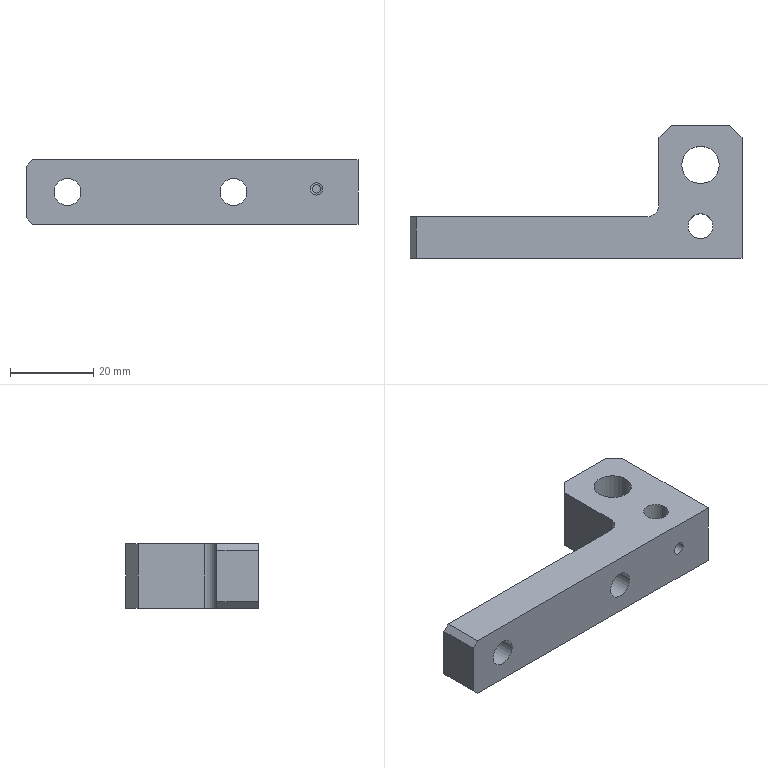NC program | NX | posted with a generic post | part box 80 x 32 x 15.5 mm
Lines 1 to 1192 of 7013:
N10 G17 G21 G94 G90
(低壁铣光面 , TOOL : D63面刀)
N12 T10 M6
N14 G53
N16 G17 G0 G90 X74.5 Y-0.25 B0. C0. S1600 M3
N18 G43 Z20. H10
N20 Z3.
N22 G94 G1 Z0. F500.
N24 X71.5
N26 X-70.
N28 X-73.
N30 Z3.
N32 G0 Z20.
N34 M5
(动态粗 , TOOL : D10-30-D10-75-3T-ROUGH)
N36 T01 M6
N38 G53
N40 G17 G0 G90 X49.529 Y17.135 B0. C0. S3500 M3
N42 G43 Z20. H1
N44 Z-16.
N46 G94 G1 X49.504 Y17.136 Z-16.156 F1500.
N48 X49.479 Y17.137 Z-16.218
N50 X49.454 Y17.138 Z-16.263
N52 X49.429 Y17.139 Z-16.3
N54 X49.404 Y17.14 Z-16.331
N56 X49.379 Y17.141 Z-16.357
N58 X49.354 Y17.142 Z-16.38
N60 X49.329 Y17.143 Z-16.4
N62 X49.305 Y17.144 Z-16.418
N64 X49.28 Y17.145 Z-16.433
N66 X49.255 Y17.146 Z-16.447
N68 X49.23 Y17.147 Z-16.458
N70 X49.205 Y17.148 Z-16.468
N72 X49.18 Y17.149 Z-16.477
N74 X49.155 Y17.15 Z-16.484
N76 X49.13 Y17.151 Z-16.49
N78 X49.105 Y17.152 Z-16.494
N80 X49.08 Y17.153 Z-16.497
N82 X49.055 Y17.154 Z-16.499
N84 X49.03 Y17.155 Z-16.5
N86 X47.521 Y17.216
N88 G3 X46.507 Y16.479 R1.01
N90 X46.179 Y13.663 R12.751
N92 X46.1 Y4.097 R320.714
N94 G1 X46.098 Y-15.673
N96 G2 X43.85 Y-19.903 R5.618
N98 X39.544 Y-21.688 R9.505
N100 X34.193 Y-22.069 R34.695
N102 G1 X25.223 Y-22.1
N104 X-39.68 Y-22.099
N106 G2 X-43.908 Y-19.844 R5.625
N108 X-45.68 Y-15.596 R9.465
N110 X-46.071 Y-10.096 R34.77
N112 G1 X-46.099 Y-1.936
N114 X-46.097 Y15.703
N116 G2 X-43.755 Y19.978 R5.656
N118 X-39.514 Y21.694 R9.606
N120 X-33.863 Y22.074 R36.888
N122 G1 X-25.883 Y22.1
N124 X39.673 Y22.099
N126 G2 X43.802 Y19.844 R5.332
N128 X45.404 Y15.68 R9.149
N130 X45.691 Y10.203 R39.744
N132 G1 X45.7 Y6.663
N134 X45.699 Y-13.747
N136 G2 X42.346 Y-19.627 R7.079
N138 X37.507 Y-21.314 R11.988
N140 X31.132 Y-21.676 R48.559
N142 G1 X22.612 Y-21.7
N144 X-37.812 Y-21.697
N146 G2 X-43.646 Y-18.316 R7.086
N148 X-45.315 Y-13.506 R12.018
N150 X-45.678 Y-7.101 R48.681
N152 G1 X-45.699 Y0.549
N154 X-45.698 Y13.752
N156 G2 X-45.105 Y16.521 R7.727
N158 G1 X-45.051 Y17.006
N160 G2 X-44.281 Y18.862 R5.993
N162 X-42.86 Y20.283 R5.993
N164 X-40.234 Y21.176 R6.013
N166 X-32.546 Y21.67 R56.619
N168 G1 X-23.306 Y21.7
N170 X37.78 Y21.698
N172 G2 X40.37 Y21.119 R7.688
N174 G1 X41.006 Y21.051
N176 G2 X42.862 Y20.281 R5.993
N178 X44.283 Y18.86 R5.993
N180 X45.051 Y17.003 R5.993
N182 X45.161 Y15.199 R13.933
N184 X45.3 Y2.158 R340.358
N186 G1 X45.298 Y-12.112
N188 G2 X41.038 Y-19.361 R8.087
N190 G3 X40.641 Y-19.642 R2.227
N192 G2 X38.969 Y-20.758 R5.996
N194 X36.999 Y-21.15 R5.998
N196 G3 X31.028 Y-21.268 R583.225
N198 G1 X19.909 Y-21.3
N200 X-36.132 Y-21.297
N202 G2 X-43.436 Y-16.904 R8.113
N204 X-44.944 Y-11.84 R14.324
N206 X-45.28 Y-4.982 R60.155
N208 G1 X-45.299 Y2.188
N210 G2 X-45.283 Y12.967 R826.898
N212 G1 X-45.15 Y14.009
N214 Y16.001
N216 X-45.088 Y16.628
N218 X-45.15 Y16.001
N220 X-45.135 Y5.721
N222 G2 X-45.046 Y-3.838 R311.792
N224 G3 X-44.74 Y-11.208 R70.008
N226 X-43.351 Y-16.213 R14.617
N228 X-37.174 Y-20.702 R8.335
N230 X-32.481 Y-21.039 R28.708
N232 G1 X-26.211 Y-21.059
N234 X22.07
N236 X22.999 Y-21.15
N238 X36.079
N240 X22.999
N242 G2 X21.258 Y-20.897 R11.67
N244 G3 X16.241 Y-20.675 R44.17
N246 G1 X10.786 Y-20.66
N248 X-28.193 Y-20.658
N250 G2 X-34.79 Y-20.519 R92.602
N252 X-39.263 Y-19.28 R10.577
N254 X-43.291 Y-14.44 R9.438
N256 X-44.442 Y-8.847 R19.304
N258 X-44.654 Y-0.722 R116.334
N260 G3 X-44.706 Y3.85 R206.056
N262 G1 X-44.754 Y4.023
N264 G3 X-45.273 Y4.483 R1.005
N266 G1 X-45.732 Y4.662
N268 X-47.582 Y5.383 Z-16.4
N270 X-47.899 Y5.509 F15000.
N272 X-48.222 Y5.62
N274 G3 X-49.223 Y4.023 R1.
N276 G1 X-49.073 Y3.834
N278 X-48.914 Y3.653
N280 G3 X-47.339 Y3.945 R1.
N282 X-47.226 Y4.528 Z-16.43 R1.395 F1500.
N284 G1 X-47.146 Y5.912 Z-16.5
N286 G2 X-45.15 Y6.001 R1.001
N288 G3 X-44.71 Y3.921 R5.882
N290 G2 X-44.455 Y1.05 R14.418
N292 G3 X-44.284 Y-7.293 R307.912
N294 X-43.446 Y-12.948 R24.348
N296 X-40.307 Y-17.939 R10.066
N298 X-35.338 Y-20.053 R10.309
N300 X-29.985 Y-20.399 R36.221
N302 G1 X-23.445 Y-20.419
N304 X11.655 Y-20.42
N306 G2 X19.874 Y-20.555 R139.074
N308 X20.938 Y-20.711 R3.882
N310 X21.501 Y-21.494 R1.001
N312 G1 X21.51 Y-22.193 Z-16.465
N314 X21.504 Y-22.891 Z-16.43
N316 X21.503 Y-23.48 Z-16.4
N318 X21.5 Y-24.334 F15000.
N320 G2 X19.782 Y-25.027 R1.
N322 X19.475 Y-24.65 R1.514
N324 X20.208 Y-23.202 R1.
N326 G1 X20.399 Y-23.172
N328 X21.805 Y-22.947 Z-16.472 F1500.
N330 G3 X22.292 Y-22.683 Z-16.5 R1.007
N332 X21.879 Y-21.016 R1.
N334 G2 X20.527 Y-20.538 R9.594
N336 G3 X17.253 Y-20.121 R14.753
N338 X8.326 Y-20.02 R234.084
N340 G1 X-25.433 Y-20.018
N342 G2 X-32.93 Y-19.866 R108.821
N344 X-37.64 Y-18.766 R13.543
N346 X-42.492 Y-13.532 R9.786
N348 X-43.757 Y-7.844 R19.136
N350 X-44.033 Y-0.181 R114.116
N352 G3 X-44.267 Y3.077 R19.89
N354 G1 X-44.758 Y4.031
N356 G2 X-44.183 Y2.873 R7.563
N358 X-43.832 Y-0.172 R14.322
N360 G3 X-43.561 Y-7.037 R185.699
N362 X-42.436 Y-12.729 R20.594
N364 X-35.221 Y-19.121 R9.98
N366 X-29.836 Y-19.724 R25.267
N368 X-21.556 Y-19.779 R473.883
N370 G1 X9.135 Y-19.78
N372 G2 X17.755 Y-19.932 R144.812
N374 X20.182 Y-20.305 R10.087
N376 G1 X20.817 Y-20.644
N378 G3 X17.878 Y-19.679 R6.566
N380 X11.531 Y-19.396 R58.748
N382 G1 X4.367 Y-19.379
N384 X-23.423 Y-19.378
N386 G2 X-31.34 Y-19.22 R119.591
N388 X-36.333 Y-18.143 R15.649
N390 X-41.825 Y-12.401 R10.299
N392 X-43.112 Y-6.533 R20.226
N394 X-43.448 Y-0.141 R193.703
N396 G3 X-43.838 Y2.531 R11.31
N398 X-44.283 Y3.14 R2.92
N400 G2 X-43.515 Y1.592 R2.753
N402 X-43.135 Y-2.133 R25.534
N404 G3 X-42.61 Y-8.337 R55.995
N406 X-40.651 Y-13.876 R14.683
N408 X-34.367 Y-18.362 R10.479
N410 X-28.813 Y-19.064 R24.602
N412 X-19.244 Y-19.139 R349.243
N414 G1 X7.124 Y-19.141
N416 G2 X16.197 Y-19.307 R150.755
N418 X19.524 Y-19.871 R12.732
N420 X20.138 Y-20.281 R1.907
N422 G3 X18.149 Y-19.315 R3.943
N424 X13.441 Y-18.828 R25.953
N426 X3.886 Y-18.74 R339.674
N428 G1 X-21.563 Y-18.738
N430 G2 X-29.84 Y-18.581 R133.457
N432 X-35.085 Y-17.531 R17.572
N434 X-41.117 Y-11.444 R10.746
N436 X-42.431 Y-5.763 R20.533
N438 X-42.872 Y-0.405 R803.758
N440 G3 X-43.387 Y2.048 R9.112
N442 G1 X-43.564 Y2.289
N444 G3 X-44.594 Y2.529 R1.042
N446 G1 X-46.531 Y2.09 Z-16.4
N448 X-46.868 Y2.011 F15000.
N450 X-47.209 Y1.948
N452 G2 X-48.032 Y2.289 R1.002
N454 G1 X-48.264 Y2.552
N456 X-48.483 Y2.825
N458 G2 X-47.455 Y4.341 R1.
N460 G1 X-47.206 Y4.262 Z-16.413 F1500.
N462 X-46.967 Y4.156 Z-16.426
N464 X-45.628 Y3.568 Z-16.5
N466 X-44.906 Y3.255
N468 G2 X-44.047 Y2.825 R4.396
N470 G1 X-43.389 Y2.093
N472 G2 X-42.753 Y-0.069 R6.385
N474 X-42.258 Y-4.978 R107.127
N476 G3 X-41.023 Y-10.769 R22.332
N478 X-33.317 Y-17.682 R11.018
N480 X-27.826 Y-18.406 R25.047
N482 X-17.597 Y-18.499 R299.997
N484 G1 X5.473 Y-18.501
N486 G2 X14.882 Y-18.678 R156.662
N488 X18.654 Y-19.291 R15.775
N490 X19.344 Y-19.628 R2.2
N492 X18.097 Y-21.176 R1.
N494 G1 X18.036 Y-21.137
N496 X17.298 Y-20.659 Z-16.456
N498 X16.553 Y-20.194 Z-16.411
N500 X16.338 Y-20.117 Z-16.4
N502 G3 X15.475 Y-21.862 R1. F15000.
N504 G1 X15.702 Y-22.052
N506 X15.938 Y-22.233
N508 G3 X16.722 Y-22.349 R1.003
N510 G1 X18.22 Y-21.951
N512 X19.386 Y-21.636 Z-16.461 F1500.
N514 G3 X19.957 Y-21.139 Z-16.5 R1.
N516 X19.697 Y-19.919 R1.
N518 X18.661 Y-19.171 R4.485
N520 X15.311 Y-18.402 R11.241
N522 X7.848 Y-18.114 R80.234
N524 G1 X0.677 Y-18.099
N526 X-19.883 Y-18.097
N528 G2 X-28.58 Y-17.934 R141.007
N530 X-34.01 Y-16.876 R18.882
N532 X-40.463 Y-10.422 R11.196
N534 X-41.791 Y-4.864 R21.95
N536 G3 X-42.388 Y-0.161 R91.366
N538 X-43.028 Y1.816 R5.976
N540 X-43.587 Y2.314 R4.524
N542 G2 X-42.849 Y1.58 R2.667
N544 X-42.07 Y-1.034 R8.377
N546 G3 X-41.335 Y-6.151 R387.917
N548 X-39.407 Y-11.769 R16.71
N550 X-32.495 Y-16.959 R11.377
N552 X-26.802 Y-17.752 R25.14
N554 X-15.913 Y-17.859 R287.99
N556 G1 X3.554 Y-17.861
N558 G2 X13.389 Y-18.026 R185.056
N560 X17.783 Y-18.681 R19.32
N562 X18.924 Y-19.207 R3.637
N564 G1 X19.263 Y-19.547
N566 G3 X17.227 Y-18.314 R3.927
N568 X12.63 Y-17.636 R20.869
N570 X2.593 Y-17.461 R186.992
N572 G1 X-15.593 Y-17.459
N574 G2 X-26.302 Y-17.352 R281.54
N576 X-32.136 Y-16.508 R24.315
N578 X-39.806 Y-9.474 R11.652
N580 X-41.197 Y-3.989 R24.621
N582 G3 X-41.984 Y0.126 R34.438
N584 X-42.614 Y1.525 R4.032
N586 G1 X-42.772 Y1.663
N588 G3 X-43.459 Y1.832 R1.005
N590 G1 X-44.18 Y1.745
N592 X-46.151 Y1.506 Z-16.4
N594 X-46.639 Y1.456 F15000.
N596 G2 X-47.24 Y1.663 R1.008
N598 G1 X-47.475 Y1.841
N600 X-47.701 Y2.031
N602 G2 X-47.262 Y3.686 R1.
N604 X-46.458 Y3.583 Z-16.442 R1.058 F1500.
N606 G1 X-45.421 Y3.08 Z-16.5
N608 X-43.321 Y2.06
N610 G2 X-42.564 Y1.502 R13.115
N612 X-41.688 Y-0.423 R5.199
N614 X-40.832 Y-4.69 R54.132
N616 G3 X-39.093 Y-10.224 R20.227
N618 X-31.63 Y-16.263 R11.763
N620 X-25.822 Y-17.099 R25.463
N622 X-16.944 Y-17.218 R214.185
N624 G1 X-0.642 Y-17.219
N626 G2 X11.503 Y-17.35 R310.505
N628 X16.681 Y-17.983 R26.207
N630 X18.406 Y-18.691 R5.341
N632 G1 X18.81 Y-19.093
N634 G3 X16.609 Y-17.743 R4.263
N636 X11.998 Y-17.027 R21.113
N638 X2.17 Y-16.823 R164.045
N640 G1 X-1.783 Y-16.819
N642 X-16.673 Y-16.818
N644 G2 X-26.031 Y-16.659 R168.413
N646 X-31.861 Y-15.624 R21.798
N648 X-39.07 Y-8.784 R12.012
N650 X-40.598 Y-3.488 R27.341
N652 G3 X-41.581 Y0.221 R22.618
N654 X-42.296 Y1.398 R3.094
N656 G1 X-42.833 Y1.703
N658 G2 X-41.604 Y0.502 R2.22
N660 X-40.545 Y-2.76 R14.77
N662 G3 X-39.179 Y-7.69 R38.632
N664 X-34.868 Y-13.598 R12.734
N666 X-28.809 Y-16.033 R14.263
N668 X-22.055 Y-16.539 R43.997
N670 X-12.875 Y-16.579 R675.537
N672 G1 X0.015 Y-16.58
N674 G2 X11.212 Y-16.754 R220.786
N676 X16.276 Y-17.466 R23.973
N678 X17.887 Y-18.17 R5.071
N680 G1 X18.29 Y-18.573
N682 G3 X16.014 Y-17.168 R4.462
N684 X11.099 Y-16.396 R22.068
N686 X0.611 Y-16.182 R173.988
N688 G1 X-3.523 Y-16.179
N690 X-15.413 Y-16.177
N692 G2 X-24.92 Y-16.017 R173.951
N694 X-30.846 Y-14.997 R23.003
N696 X-38.344 Y-8.143 R12.438
N698 X-39.883 Y-3.596 R28.44
N700 G3 X-41.077 Y0.053 R22.128
N702 X-41.845 Y1.168 R3.012
N704 G1 X-41.947 Y1.232
N706 G3 X-42.706 Y1.216 R1.003
N708 G1 X-43.141 Y1.026
N710 X-44.961 Y0.233 Z-16.4
N712 X-45.246 Y0.105 F15000.
N714 X-45.537 Y-0.006
N716 G2 X-46.262 Y0.075 R1.004
N718 G1 X-46.537 Y0.217
N720 X-46.802 Y0.374
N722 G2 X-46.562 Y2.111 R1.
N724 X-45.934 Y2.144 Z-16.432 R1.09 F1500.
N726 G1 X-44.608 Y1.904 Z-16.5
N728 X-43.578 Y1.722
N730 X-42.55 Y1.527
N732 G2 X-41.633 Y1.014 R3.108
N734 X-40.472 Y-1.044 R5.989
N736 X-39.162 Y-5.207 R99.726
N738 G3 X-36.535 Y-10.506 R17.1
N740 X-29.674 Y-14.973 R12.719
N742 X-23.505 Y-15.819 R28.09
N744 X-13.097 Y-15.938 R263.064
N746 G1 X-3.582 Y-15.939
N748 G2 X9.298 Y-16.07 R351.893
N750 X15.062 Y-16.722 R31.958
N752 X17.292 Y-17.58 R7.102
N754 G1 X17.74 Y-18.023
N756 G3 X15.46 Y-16.597 R4.547
N758 X10.749 Y-15.801 R21.24
N760 X1.173 Y-15.547 R138.744
N762 G1 X-4.933 Y-15.539
N764 G2 X-21.473 Y-15.475 R901.197
N766 X-28.064 Y-14.848 R37.192
N768 X-34.475 Y-11.77 R13.696
N770 X-38.204 Y-6.278 R14.658
N772 X-39.789 Y-1.837 R109.532
N774 G3 X-41.126 Y0.742 R8.722
N776 X-41.659 Y1.148 R1.357
N778 X-42.293 Y1.129 R1.008
N780 G1 X-43.026 Y0.86
N782 X-44.89 Y0.175 Z-16.4
N784 X-45.175 Y0.069 F15000.
N786 X-45.464 Y-0.027
N788 G2 X-45.975 Y-0.009 R1.018
N790 G1 X-46.202 Y0.06
N792 X-46.426 Y0.139
N794 G2 X-46.466 Y1.927 R1.
N796 X-45.708 Y2.005 Z-16.439 R1.059 F1500.
N798 G1 X-44.526 Y1.765 Z-16.5
N800 X-42.064 Y1.266
N802 G2 X-40.769 Y0.404 R1.908
N804 X-39.4 Y-2.364 R11.415
N806 G3 X-37.633 Y-6.861 R53.005
N808 X-32.632 Y-12.664 R13.505
N810 X-26.586 Y-14.787 R16.008
N812 X-19.378 Y-15.264 R51.827
N814 X-4.992 Y-15.299 R934.072
N816 G2 X8.312 Y-15.432 R368.323
N818 X14.307 Y-16.094 R34.116
N820 X16.716 Y-17.006 R7.636
N822 G1 X17.207 Y-17.49
N824 G3 X14.832 Y-15.996 R4.732
N826 X9.831 Y-15.161 R22.346
N828 X-0.444 Y-14.905 R152.646
N830 G1 X-10.223 Y-14.899
N832 G2 X-21.892 Y-14.782 R312.697
N834 X-28.185 Y-13.952 R29.575
N836 X-36.83 Y-7.167 R13.458
N838 X-38.88 Y-2.571 R41.643
N840 G3 X-40.422 Y0.348 R12.502
N842 X-41.639 Y1.142 R1.826
N844 G2 X-40.2 Y0.201 R2.235
N846 X-38.682 Y-2.546 R12.74
N848 G3 X-36.597 Y-6.976 R44.506
N850 X-27.684 Y-13.727 R13.786
N852 X-21.357 Y-14.539 R31.088
N854 X-9.688 Y-14.659 R312.753
N856 G2 X6.179 Y-14.751 R662.708
N858 X12.93 Y-15.333 R45.515
N860 X16.105 Y-16.396 R9.681
N862 G1 X16.634 Y-16.917
N864 G3 X15.883 Y-16.173 R7.843
N866 X13.019 Y-15.067 R8.132
N868 X6.614 Y-14.391 R37.753
N870 X-6.164 Y-14.26 R369.433
N872 G2 X-20.223 Y-14.166 R508.192
N874 X-26.889 Y-13.411 R34.152
N876 X-36.141 Y-6.634 R14.127
N878 X-38.302 Y-2.394 R50.797
N880 G3 X-39.977 Y0.318 R11.844
N882 X-40.872 Y0.934 R1.709
N884 X-41.657 Y0.725 R1.002
N886 G1 X-41.947 Y0.491
N888 X-43.492 Y-0.756 Z-16.4
N890 X-43.759 Y-0.976 F15000.
N892 X-44.036 Y-1.181
N894 G2 X-44.742 Y-1.3 R1.005
N896 G1 X-45.133 Y-1.21
N898 G2 X-45.361 Y0.555 R1.
N900 X-44.784 Y0.736 Z-16.431 R1.097 F1500.
N902 G1 X-43.417 Y0.856 Z-16.5
N904 X-41.501 Y1.024
N906 G2 X-40.56 Y0.85 R3.917
N908 X-39.073 Y-0.687 R4.537
N910 X-37.162 Y-4.224 R37.193
N912 G3 X-33.985 Y-8.986 R20.201
N914 X-26.57 Y-13.143 R14.52
N916 X-19.966 Y-13.914 R34.232
N918 X-9.107 Y-14.019 R338.578
N920 G2 X5.684 Y-14.126 R537.149
N922 X12.534 Y-14.767 R43.195
N924 X15.656 Y-15.878 R9.3
N926 X16.194 Y-16.441 R2.248
N928 G3 X14.273 Y-15.016 R3.877
N930 X9.73 Y-14.029 R17.716
N932 X1.229 Y-13.649 R91.306
N934 G1 X-11.945 Y-13.615
N936 G2 X-21.511 Y-13.406 R149.052
N938 X-27.835 Y-12.242 R24.504
N940 X-35.385 Y-6.253 R14.709
N942 X-37.802 Y-2.091 R65.875
N944 G3 X-39.657 Y0.432 R10.343
N946 X-40.886 Y0.937 R1.619
N948 G2 X-39.451 Y0.348 R1.943
N950 X-37.587 Y-2.096 R10.604
N952 G3 X-35.075 Y-6.202 R64.815
N954 X-25.684 Y-12.508 R15.159
N956 X-18.898 Y-13.277 R35.917
N958 X-5.565 Y-13.38 R445.561
N960 G2 X6.897 Y-13.579 R248.379
N962 X12.765 Y-14.346 R31.581
N964 X15.459 Y-15.519 R7.409
N966 G1 X15.654 Y-15.746
N968 G2 X15.191 Y-17.183 R1.
N970 X14.279 Y-17.123 Z-16.452 R1.043
N972 G1 X13.343 Y-16.671 Z-16.4
N974 X13.132 Y-16.568 F15000.
N976 X12.915 Y-16.477
N978 G3 X11.785 Y-17.98 R1.
N980 X12.094 Y-18.378 R1.708
N982 X13.165 Y-18.524 R1.001
N984 G1 X14.245 Y-18.021
N986 X15.484 Y-17.438 Z-16.469 F1500.
N988 G3 X15.902 Y-17. Z-16.5 R1.003
N990 X15.775 Y-15.931 R1.001
N992 X15.35 Y-15.347 R3.069
N994 X12.903 Y-14.121 R6.419
N996 X7.361 Y-13.248 R26.487
N998 X-3.534 Y-12.985 R169.805
N1000 G2 X-18.046 Y-12.891 R614.066
N1002 X-24.96 Y-12.173 R38.405
N1004 X-34.638 Y-5.881 R15.562
N1006 X-37.316 Y-1.798 R90.835
N1008 G3 X-39.308 Y0.52 R9.395
N1010 X-39.999 Y0.85 R1.494
N1012 X-40.579 Y0.664 R1.008
N1014 G1 X-41.338 Y0.121
N1016 X-42.953 Y-1.034 Z-16.4
N1018 X-43.311 Y-1.277 F15000.
N1020 G2 X-43.868 Y-1.384 R1.011
N1022 G1 X-44.148 Y-1.358
N1024 X-44.425 Y-1.318
N1026 G2 X-44.991 Y0.236 R1.
N1028 X-44.154 Y0.655 Z-16.449 R1.041 F1500.
N1030 G1 X-43.142 Y0.722 Z-16.5
N1032 X-40.573 Y0.893
N1034 G2 X-39.497 Y0.698 R2.364
N1036 X-37.662 Y-1.033 R6.257
N1038 X-35.207 Y-4.625 R94.593
N1040 G3 X-30.576 Y-9.436 R18.074
N1042 X-23.73 Y-12.095 R17.272
N1044 X-16.441 Y-12.68 R48.322
N1046 X-2.465 Y-12.75 R889.617
N1048 G2 X7.763 Y-13.057 R138.301
N1050 X13.109 Y-14.002 R23.63
N1052 X15.341 Y-15.214 R5.821
N1054 X15.61 Y-15.659 R6.786
N1056 G3 X14.259 Y-14.283 R2.844
N1058 X10.349 Y-13.044 R12.457
N1060 X2.675 Y-12.429 R54.961
N1062 X-13.159 Y-12.32 R926.974
N1064 G2 X-21.547 Y-11.951 R81.189
N1066 X-28.21 Y-10.157 R20.54
N1068 X-34.066 Y-5.305 R16.741
N1070 X-36.801 Y-1.567 R175.291
N1072 G3 X-38.938 Y0.599 R8.888
N1074 X-40.001 Y0.85 R1.565
N1076 G2 X-38.536 Y0.415 R1.974
N1078 X-36.396 Y-1.802 R10.634
N1080 G3 X-33.398 Y-5.676 R76.911
N1082 X-23.65 Y-11.31 R16.856
N1084 X-16.553 Y-12.011 R41.802
N1086 X-2.682 Y-12.114 R672.505
N1088 G2 X7.185 Y-12.433 R131.92
N1090 X12.679 Y-13.42 R24.206
N1092 X15.088 Y-14.748 R6.268
N1094 G1 X15.229 Y-14.942
N1096 G2 X14.234 Y-16.311 R1.
N1098 X13.523 Y-15.949 Z-16.459 R1.06
N1100 G1 X12.701 Y-15.122 Z-16.4
N1102 X12.551 Y-14.972 F15000.
N1104 X12.394 Y-14.829
N1106 G3 X10.913 Y-16.098 R1.
N1108 G1 X11.024 Y-16.31
N1110 X11.146 Y-16.517
N1112 G3 X12.039 Y-16.923 R1.001
N1114 G1 X13.379 Y-16.807
N1116 X14.022 Y-16.755 Z-16.433 F1500.
N1118 X14.664 Y-16.691 Z-16.465
N1120 G3 X15.259 Y-16.361 Z-16.5 R1.001
N1122 X15.384 Y-15.236 R1.
N1124 X14.139 Y-13.863 R2.761
N1126 X10.377 Y-12.533 R11.522
N1128 X3.006 Y-11.825 R47.399
N1130 X-10.703 Y-11.69 R482.242
N1132 G2 X-19.876 Y-11.395 R110.821
N1134 X-26.701 Y-9.867 R23.496
N1136 X-33.296 Y-5.001 R17.49
N1138 X-36.235 Y-1.397 R237.717
N1140 G3 X-38.443 Y0.622 R9.141
N1142 X-39.566 Y0.85 R1.771
N1144 G2 X-37.927 Y0.388 R2.25
N1146 X-35.449 Y-2.043 R12.846
N1148 G3 X-32.027 Y-5.933 R48.674
N1150 X-22.778 Y-10.686 R17.754
N1152 X-15.409 Y-11.378 R44.665
N1154 X-1.744 Y-11.489 R940.968
N1156 G2 X7.483 Y-11.892 R101.976
N1158 X12.699 Y-12.989 R21.196
N1160 X14.974 Y-14.404 R5.746
N1162 X15.172 Y-14.738 R3.708
N1164 X14.316 Y-16.022 R1.
N1166 X13.49 Y-15.723 Z-16.454 R1.048
N1168 G1 X12.67 Y-15.022 Z-16.4
N1170 X12.509 Y-14.885 F15000.
N1172 X12.341 Y-14.756
N1174 G3 X10.856 Y-15.895 R1.
N1176 G1 X10.98 Y-16.267
N1178 G3 X12.116 Y-16.808 R1.
N1180 G1 X13.235 Y-16.54
N1182 X14.582 Y-16.212 Z-16.47 F1500.
N1184 G3 X15.069 Y-15.879 Z-16.5 R1.004
N1186 X15.242 Y-14.969 R1.001
N1188 X14.33 Y-13.656 R2.177
N1190 X11.153 Y-12.216 R9.087
N1192 X4.765 Y-11.308 R32.986
N1194 X-6.209 Y-11.064 R198.718
N1196 G2 X-17.336 Y-10.879 R228.306
N1198 X-24.376 Y-9.791 R30.817
N1200 X-32.466 Y-4.755 R18.239
N1202 X-35.632 Y-1.251 R246.669
N1204 G3 X-37.938 Y0.664 R9.421
N1206 X-38.522 Y0.85 R1.517
N1208 G1 X-39.032
N1210 G2 X-37.249 Y0.351 R2.499
N1212 X-34.639 Y-2.044 R14.913
N1214 G3 X-30.875 Y-5.866 R43.368
N1216 X-21.861 Y-10.074 R18.805
N1218 X-14.248 Y-10.745 R48.189
N1220 X-1.815 Y-10.858 R967.096
N1222 G2 X7.336 Y-11.312 R92.817
N1224 X12.491 Y-12.47 R20.622
N1226 X14.794 Y-13.939 R6.086
N1228 X15.14 Y-14.635 R1.475
N1230 G3 X14.159 Y-13.179 R2.428
N1232 X10.76 Y-11.619 R9.477
N1234 X4.416 Y-10.692 R33.274
N1236 X-7.025 Y-10.422 R195.685
N1238 G2 X-17.191 Y-10.194 R171.131
N1240 X-24.409 Y-8.915 R28.924
N1242 X-31.849 Y-4.288 R19.543
N1244 G1 X-35.068 Y-1.045
N1246 G3 X-37.519 Y0.764 R9.005
N1248 X-38.464 Y0.85 R2.426
N1250 G2 X-37.397 Y0.756 R2.919
N1252 X-35.086 Y-0.798 R7.692
N1254 X-31.581 Y-4.18 R693.236
N1256 G3 X-20.648 Y-9.516 R20.226
N1258 X-12.758 Y-10.12 R55.393
N1260 G1 X-2.154 Y-10.225
N1262 G2 X7.182 Y-10.732 R87.654
N1264 X12.407 Y-11.994 R19.933
N1266 X14.735 Y-13.595 R5.927
N1268 X14.947 Y-13.989 R1.907
N1270 X14.232 Y-15.056 R1.
N1272 X13.292 Y-14.852 Z-16.45 R1.043
N1274 G1 X12.491 Y-14.28 Z-16.4
N1276 X12.27 Y-14.121 F15000.
N1278 X12.041 Y-13.973
N1280 G3 X10.631 Y-15.145 R1.
N1282 X10.822 Y-15.637 R1.659
N1284 X11.893 Y-16.054 R1.
N1286 G1 X12.882 Y-15.811
N1288 X14.355 Y-15.445 Z-16.476 F1500.
N1290 G3 X14.753 Y-15.208 Z-16.5 R1.013
N1292 X15.01 Y-14.204 R1.001
N1294 X14.134 Y-12.807 R2.323
N1296 X10.832 Y-11.149 R9.025
N1298 X4.687 Y-10.123 R30.176
N1300 X-6.255 Y-9.788 R156.948
N1302 G2 X-16.36 Y-9.555 R178.879
N1304 X-23.674 Y-8.294 R30.281
N1306 X-31.275 Y-3.8 R20.932
N1308 G3 X-34.808 Y-0.569 R196.686
N1310 X-37.012 Y0.821 R7.399
N1312 X-37.849 Y0.85 R5.085
N1314 G2 X-36.724 Y0.761 R3.284
N1316 X-34.307 Y-0.769 R8.356
N1318 G3 X-30.628 Y-4.01 R735.547
N1320 X-19.783 Y-8.897 R21.419
N1322 X-11.621 Y-9.486 R59.656
N1324 G2 X0.548 Y-9.667 R843.675
N1326 X8.545 Y-10.397 R54.954
N1328 X13.041 Y-11.876 R14.896
N1330 X14.834 Y-13.488 R4.534
N1332 G1 X14.925 Y-13.773
N1334 G2 X14.272 Y-14.851 R1.
N1336 X13.335 Y-14.715 Z-16.45 R1.039
N1338 G1 X12.481 Y-14.192 Z-16.4
N1340 X12.242 Y-14.043 F15000.
N1342 X11.995 Y-13.907
N1344 G3 X10.609 Y-14.93 R1.
N1346 X10.711 Y-15.458 R1.674
N1348 X12.008 Y-15.983 R1.
N1350 G1 X12.825 Y-15.647
N1352 X14.387 Y-15. Z-16.485 F1500.
N1354 X14.515 Y-14.926 Z-16.493
N1356 X14.631 Y-14.836 Z-16.5
N1358 G3 X14.949 Y-14.003 R1.002
N1360 X14.331 Y-12.643 R1.93
N1362 X11.45 Y-10.878 R7.613
N1364 X5.676 Y-9.638 R24.149
N1366 X-4.181 Y-9.174 R105.587
N1368 G2 X-14.842 Y-8.959 R274.169
N1370 X-22.366 Y-7.85 R34.645
N1372 X-30.544 Y-3.454 R22.119
N1374 G3 X-34.246 Y-0.363 R152.482
N1376 X-36.313 Y0.828 R7.324
N1378 X-37.148 Y0.85 R12.288
N1380 G2 X-35.99 Y0.763 R3.507
N1382 X-33.551 Y-0.683 R8.938
N1384 G3 X-29.552 Y-3.896 R248.844
N1386 X-18.868 Y-8.288 R22.742
N1388 X-10.583 Y-8.852 R64.609
N1390 G2 X1.101 Y-9.076 R466.336
N1392 X8.818 Y-9.921 R47.516
N1394 X13.125 Y-11.505 R13.811
N1396 X14.83 Y-13.203 R4.353
N1398 X14.919 Y-13.702 R2.812
N1400 G3 X14.257 Y-12.201 R2.127
N1402 X11.331 Y-10.357 R7.793
N1404 X5.548 Y-9.052 R23.828
N1406 X-3.988 Y-8.545 R97.24
N1408 G2 X-14.105 Y-8.317 R282.011
N1410 X-21.779 Y-7.194 R35.91
N1412 X-30. Y-2.961 R23.799
N1414 G3 X-33.651 Y-0.17 R104.81
N1416 X-35.552 Y0.833 R7.146
N1418 G1 X-36.421 Y0.85
N1420 G2 X-35.332 Y0.802 R4.677
N1422 X-32.879 Y-0.506 R8.52
N1424 G3 X-28.681 Y-3.593 R282.208
N1426 X-17.795 Y-7.702 R24.327
N1428 X-9.326 Y-8.225 R73.001
N1430 G2 X1.959 Y-8.515 R271.629
N1432 X9.238 Y-9.496 R40.228
N1434 X13.35 Y-11.234 R12.442
N1436 X14.817 Y-12.888 R4.005
N1438 G1 X14.882 Y-13.325
N1440 G3 X14.232 Y-11.794 R2.217
N1442 X11.326 Y-9.876 R7.824
N1444 X5.743 Y-8.508 R22.699
N1446 X-3.267 Y-7.931 R83.618
N1448 G2 X-13.49 Y-7.67 R321.822
N1450 X-21.339 Y-6.504 R36.718
N1452 X-29.319 Y-2.577 R25.533
N1454 G3 X-33.118 Y0.072 R77.743
N1456 X-34.771 Y0.843 R5.78
N1458 G1 X-35.641 Y0.85
N1460 G2 X-34.485 Y0.803 R5.227
N1462 X-31.944 Y-0.479 R9.322
N1464 G3 X-27.496 Y-3.464 R141.426
N1466 X-16.814 Y-7.102 R26.006
N1468 X-8.522 Y-7.592 R79.304
N1470 G2 X2.211 Y-7.932 R216.085
N1472 X9.407 Y-9.024 R37.11
N1474 X13.457 Y-10.892 R11.844
N1476 X14.818 Y-12.578 R3.858
N1478 G1 X14.85 Y-12.999
N1480 G3 X14.372 Y-11.576 R1.969
N1482 X11.618 Y-9.527 R7.219
N1484 X6.174 Y-8.008 R20.613
N1486 X-2.787 Y-7.318 R72.546
N1488 G2 X-12.758 Y-7.032 R389.64
N1490 X-20.874 Y-5.829 R38.082
N1492 X-28.611 Y-2.206 R27.445
N1494 G3 X-32.53 Y0.282 R62.804
N1496 X-33.903 Y0.847 R4.814
N1498 G1 X-34.789 Y0.85
N1500 G2 X-33.572 Y0.804 R5.743
N1502 X-30.89 Y-0.482 R10.437
N1504 G3 X-26.059 Y-3.417 R88.162
N1506 X-15.744 Y-6.511 R28.031
N1508 X-7.21 Y-6.974 R92.939
N1510 G2 X3.022 Y-7.404 R152.895
N1512 X9.799 Y-8.627 R32.355
N1514 X13.58 Y-10.564 R11.087
N1516 X14.83 Y-12.269 R3.695
N1518 G1 X14.85 Y-12.691
N1520 G3 X14.285 Y-11.053 R2.21
N1522 X11.378 Y-8.934 R7.772
N1524 X5.733 Y-7.377 R21.639
N1526 X-2.982 Y-6.687 R73.389
N1528 G2 X-12.628 Y-6.359 R314.193
N1530 X-20.874 Y-5.028 R37.318
N1532 X-28.099 Y-1.712 R30.487
N1534 G3 X-31.9 Y0.474 R46.457
N1536 X-32.975 Y0.85 R3.53
N1538 G1 X-33.875
N1540 G2 X-32.597 Y0.807 R6.544
N1542 X-30.039 Y-0.321 R10.758
N1544 G3 X-25.103 Y-3.063 R91.763
N1546 X-14.974 Y-5.886 R29.972
N1548 X-6.979 Y-6.337 R96.01
N1550 G2 X3.044 Y-6.818 R141.005
N1552 X9.828 Y-8.126 R31.342
N1554 X13.613 Y-10.156 R11.024
N1556 X14.831 Y-11.877 R3.818
N1558 G1 X14.85 Y-12.326
N1560 G3 X14.308 Y-10.66 R2.278
N1562 X11.452 Y-8.482 R7.755
N1564 X5.875 Y-6.838 R20.947
N1566 X-2.974 Y-6.064 R69.259
N1568 G2 X-12.32 Y-5.697 R295.012
N1570 X-20.932 Y-4.211 R37.329
N1572 X-27.791 Y-1.117 R35.452
N1574 G3 X-31.41 Y0.718 R28.671
N1576 X-31.912 Y0.85 R3.068
N1578 G1 X-32.902
N1580 G2 X-31.562 Y0.812 R8.162
N1582 X-28.823 Y-0.321 R11.991
N1584 G3 X-23.485 Y-2.974 R68.377
N1586 X-13.776 Y-5.308 R32.909
N1588 X-4.964 Y-5.757 R132.445
N1590 G2 X4.469 Y-6.405 R93.136
N1592 X10.742 Y-7.965 R25.159
N1594 X14.085 Y-10.189 R9.155
N1596 X14.847 Y-11.575 R2.869
N1598 G1 X14.85 Y-11.918
N1600 G3 X14.287 Y-10.195 R2.406
N1602 X11.348 Y-7.94 R8.041
N1604 X5.58 Y-6.225 R21.495
N1606 X-3.496 Y-5.419 R71.474
N1608 G2 X-12.491 Y-4.998 R205.35
N1610 X-21.874 Y-3.095 R35.978
N1612 X-27.69 Y-0.448 R49.432
N1614 G3 X-30.669 Y0.839 R16.826
N1616 G1 X-31.836 Y0.85
N1618 G2 X-30.416 Y0.814 R9.386
N1620 X-27.787 Y-0.181 R12.695
N1622 G3 X-22.083 Y-2.725 R65.521
N1624 X-12.328 Y-4.748 R36.743
N1626 X-3.041 Y-5.201 R233.284
N1628 G2 X5.787 Y-6.046 R67.398
N1630 X11.565 Y-7.853 R20.672
N1632 X14.395 Y-10.145 R7.719
N1634 X14.85 Y-11.196 R2.29
N1636 G1 Y-11.496
N1638 G3 X14.237 Y-9.682 R2.517
N1640 X11.118 Y-7.33 R8.5
N1642 X5.162 Y-5.589 R22.589
N1644 X-3.903 Y-4.774 R74.812
N1646 G2 X-13.022 Y-4.254 R155.583
N1648 X-25.456 Y-0.812 R36.391
N1650 G3 X-29.278 Y0.805 R35.314
N1652 G1 X-29.544 Y0.85
N1654 X-30.714
N1656 G2 X-29.167 Y0.816 R11.377
N1658 X-26.176 Y-0.253 R15.658
N1660 G3 X-19.405 Y-2.807 R49.32
N1662 X-10.44 Y-4.213 R44.523
N1664 X-1.524 Y-4.661 R930.797
N1666 G2 X6.879 Y-5.712 R53.034
N1668 X12.235 Y-7.744 R17.613
N1670 X14.574 Y-9.987 R6.701
N1672 X14.85 Y-11.061 R1.712
N1674 G3 X14.261 Y-9.258 R2.544
N1676 X11.209 Y-6.873 R8.466
N1678 X5.233 Y-5.035 R22.166
N1680 X-3.312 Y-4.177 R69.219
N1682 G2 X-12.33 Y-3.631 R185.513
N1684 X-24.597 Y-0.467 R39.737
N1686 G3 X-28.056 Y0.838 R29.872
N1688 G1 X-29.466 Y0.85
N1690 G2 X-27.808 Y0.82 R15.002
N1692 X-24.686 Y-0.198 R18.058
N1694 G3 X-16.537 Y-2.737 R45.813
N1696 X-7.809 Y-3.71 R61.482
N1698 G2 X1.609 Y-4.309 R190.929
N1700 X8.989 Y-5.758 R35.018
N1702 X13.302 Y-8.039 R12.975
N1704 X14.822 Y-10.114 R4.742
N1706 X14.85 Y-10.638 R6.347
N1708 G3 X14.263 Y-8.796 R2.604
N1710 X11.219 Y-6.372 R8.562
N1712 X5.261 Y-4.474 R22.071
N1714 X-3.222 Y-3.557 R67.291
N1716 G2 X-12.207 Y-2.95 R179.048
N1718 X-23.345 Y-0.256 R42.966
N1720 G3 X-26.598 Y0.845 R30.586
N1722 G1 X-28.099 Y0.85
N1724 G2 X-26.199 Y0.808 R14.44
N1726 X-23.181 Y-0.084 R22.076
N1728 G3 X-9.502 Y-2.938 R48.167
N1730 G2 X-0.314 Y-3.528 R963.846
N1732 X7.795 Y-4.852 R43.647
N1734 X12.722 Y-7.094 R15.617
N1736 X14.737 Y-9.409 R5.877
N1738 X14.85 Y-10.176 R1.592
N1740 G3 X14.267 Y-8.328 R2.635
N1742 X11.189 Y-5.847 R8.69
N1744 X5.107 Y-3.878 R22.384
N1746 X-3.367 Y-2.923 R68.243
N1748 G2 X-12.292 Y-2.246 R160.551
N1750 X-21.873 Y-0.076 R46.874
N1752 G3 X-24.946 Y0.848 R33.794
N1754 G1 X-26.595 Y0.85
N1756 G2 X-24.469 Y0.809 R17.604
N1758 X-20.736 Y-0.191 R34.616
N1760 G3 X-8.8 Y-2.325 R53.319
N1762 G2 X0.141 Y-2.964 R454.269
N1764 X8.003 Y-4.37 R41.236
N1766 X12.902 Y-6.737 R15.123
N1768 X14.738 Y-8.942 R5.78
N1770 X14.85 Y-9.712 R1.609
N1772 G3 X14.272 Y-7.855 R2.667
N1774 X11.247 Y-5.365 R8.72
N1776 X5.13 Y-3.315 R22.253
N1778 X-3.809 Y-2.265 R70.09
N1780 G2 X-12.795 Y-1.484 R130.622
N1782 X-21.64 Y0.503 R60.796
N1784 G3 X-23.049 Y0.85 R37.323
N1786 G1 X-24.858
N1788 G2 X-22.54 Y0.817 R25.496
N1790 X-18.526 Y-0.103 R46.167
N1792 G3 X-7.206 Y-1.787 R64.195
N1794 G2 X1.941 Y-2.572 R161.133
N1796 X9.203 Y-4.238 R32.996
N1798 X13.468 Y-6.728 R12.769
N1800 X14.832 Y-8.757 R4.627
N1802 G1 X14.85 Y-9.236
N1804 G3 X14.224 Y-7.3 R2.769
N1806 X11.029 Y-4.731 R9.169
N1808 X4.914 Y-2.702 R23.118
N1810 X-3.575 Y-1.654 R69.861
N1812 G2 X-12.495 Y-0.828 R137.758
N1814 X-20.178 Y0.724 R78.525
N1816 G1 X-20.812 Y0.85
N1818 X-22.912
N1820 G2 X-20.14 Y0.81 R31.043
N1822 X-15.548 Y-0.063 R99.042
N1824 G3 X-6.144 Y-1.217 R82.703
N1826 G2 X2.911 Y-2.123 R116.019
N1828 X9.919 Y-3.995 R29.145
N1830 X13.755 Y-6.52 R11.547
N1832 X14.841 Y-8.325 R4.11
N1834 G1 X14.85 Y-8.774
N1836 G3 X14.221 Y-6.805 R2.79
N1838 X11.071 Y-4.231 R9.213
N1840 X4.751 Y-2.098 R23.359
N1842 X-3.993 Y-0.991 R73.169
N1844 G2 X-13.535 Y0.022 R120.1
N1846 X-18.117 Y0.85 R570.71
N1848 G1 X-20.637
N1850 G2 X-17.326 Y0.819 R55.276
N1852 X-12.187 Y0.073 R218.322
N1854 G3 X-2.797 Y-0.855 R185.03
N1856 G2 X5.933 Y-2.146 R59.57
N1858 X11.786 Y-4.439 R20.284
N1860 X14.471 Y-6.96 R8.068
N1862 X14.85 Y-8.267 R2.049
N1864 G3 X14.268 Y-6.373 R2.739
N1866 X11.2 Y-3.778 R9.081
N1868 X5.039 Y-1.588 R22.766
N1870 X-3.73 Y-0.383 R69.764
N1872 G2 X-14.652 Y0.85 R152.897
N1874 G1 X-17.832
N1876 G2 X-13.369 Y0.813 R80.606
N1878 G3 X-1.144 Y-0.4 R970.751
N1880 G2 X7.023 Y-1.878 R47.993
N1882 X12.422 Y-4.349 R17.724
N1884 X14.655 Y-6.804 R6.917
N1886 X14.85 Y-7.76 R1.66
N1888 G3 X14.22 Y-5.803 R2.827
N1890 X11.072 Y-3.18 R9.404
N1892 X4.805 Y-0.964 R23.496
N1894 X-3.644 Y0.239 R70.85
N1896 G1 X-9.836 Y0.85
N1898 X-14.096
N1900 G2 X-7.816 Y0.818 R177.13
N1902 X3.133 Y-0.407 R105.531
N1904 X10.13 Y-2.49 R28.48
N1906 X13.84 Y-5.103 R11.471
N1908 X14.844 Y-6.869 R3.971
N1910 G1 X14.85 Y-7.291
N1912 G3 X14.246 Y-5.33 R2.855
N1914 X11.118 Y-2.675 R9.406
N1916 X4.772 Y-0.383 R23.578
N1918 X-3.539 Y0.85 R68.334
N1920 G1 X-8.669
N1922 G2 X-1.853 Y0.827 R266.691
N1924 X8.163 Y-1.138 R39.604
N1926 X13.016 Y-3.78 R15.452
N1928 X14.8 Y-6.157 R5.807
N1930 X14.85 Y-6.784 R2.238
N1932 G3 X14.254 Y-4.831 R2.858
N1934 X11.1 Y-2.132 R9.481
N1936 X4.643 Y0.221 R23.903
N1938 X1.242 Y0.85 R49.609
N1940 G1 X-2.478
N1942 G2 X2.174 Y0.823 R102.726
N1944 X10.901 Y-1.811 R24.446
N1946 X14.171 Y-4.486 R10.093
N1948 X14.85 Y-5.92 R3.163
N1950 G1 Y-6.28
N1952 G3 X14.25 Y-4.31 R2.883
N1954 X11.124 Y-1.61 R9.535
N1956 X4.174 Y0.85 R22.538
N1958 G1 X1.684
N1960 G2 X4.776 Y0.821 R46.993
N1962 X12.509 Y-2.32 R17.593
N1964 X14.696 Y-4.865 R6.904
N1966 X14.85 Y-5.799 R1.73
N1968 G3 X14.205 Y-3.725 R2.978
N1970 X10.964 Y-0.982 R9.88
N1972 X6.214 Y0.85 R16.404
N1974 G1 X4.354
N1976 G2 X6.707 Y0.814 R23.244
N1978 X13.448 Y-2.611 R13.597
N1980 X14.834 Y-4.757 R5.011
N1982 G1 X14.85 Y-5.285
N1984 G3 X14.219 Y-3.222 R2.969
N1986 X10.929 Y-0.432 R9.812
N1988 X7.794 Y0.847 R12.224
N1990 G1 X6.306 Y0.85
N1992 G2 X8.115 Y0.821 R17.474
N1994 X12.509 Y-1.265 R10.879
N1996 X14.7 Y-3.832 R6.948
N1998 X14.85 Y-4.73 R1.694
N2000 G3 X14.239 Y-2.728 R2.927
N2002 X10.663 Y0.21 R9.56
N2004 X8.98 Y0.849 R6.141
N2006 G1 X7.851 Y0.85
N2008 G2 X9.329 Y0.814 R9.84
N2010 X14.398 Y-2.738 R8.796
N2012 X14.85 Y-3.845 R2.74
N2014 G1 Y-4.205
N2016 G3 X14.218 Y-2.175 R2.964
N2018 X10.087 Y0.835 R8.372
N2020 G1 X9.025 Y0.85
N2022 G2 X10.298 Y0.812 R7.416
N2024 X14.596 Y-2.57 R7.225
N2026 X14.85 Y-3.722 R1.907
N2028 G3 X14.2 Y-1.637 R2.973
N2030 X10.936 Y0.83 R6.816
N2032 X10.034 Y0.85 R19.761
N2034 G2 X11.256 Y0.772 R4.136
N2036 X14.715 Y-2.316 R6.01
N2038 X14.85 Y-3.169 R1.645
N2040 G3 X14.216 Y-1.168 R2.85
N2042 X11.625 Y0.831 R5.377
N2044 G1 X10.817 Y0.85
N2046 G2 X11.853 Y0.794 R3.765
N2048 X14.819 Y-2.113 R4.851
N2050 X14.85 Y-2.681 R4.408
N2052 G3 X14.166 Y-0.644 R2.78
N2054 X12.22 Y0.827 R4.222
N2056 X11.531 Y0.85 R12.456
N2058 G2 X13.417 Y0.251 R2.451
N2060 X14.838 Y-1.734 R3.81
N2062 G1 X14.85 Y-2.184
N2064 G3 X14.14 Y-0.207 R2.593
N2066 X12.68 Y0.832 R3.071
N2068 G1 X12.081 Y0.85
N2070 G2 X13.797 Y0.262 R2.115
N2072 X14.845 Y-1.355 R2.953
N2074 G1 X14.85 Y-1.714
N2076 G3 X14.113 Y0.162 R2.322
N2078 X12.985 Y0.846 R2.012
N2080 G1 X12.568 Y0.85
N2082 G2 X14.096 Y0.28 R1.802
N2084 X14.85 Y-1.033 R2.216
N2086 G1 Y-1.273
N2088 G3 X14.098 Y0.445 R2.006
N2090 X12.966 Y0.85 R1.366
N2092 G2 X14.34 Y0.289 R1.544
N2094 X14.85 Y-0.925 R1.58
N2096 G3 X13.658 Y0.834 R1.659
N2098 G1 X13.277 Y0.85
N2100 G2 X14.595 Y0.205 R1.368
N2102 X14.85 Y-0.601 R1.181
N2104 G3 X13.73 Y0.85 R1.3
N2106 G1 X13.542
N2108 G2 X14.85 Y-0.36 R1.183
N2110 G3 X13.735 Y0.85 R1.069
N2112 G2 X14.839 Y-0.065 R1.03
N2114 G3 X13.965 Y0.836 R1.008
N2116 X12.942 Y0.22 R1.
N2118 G1 X12.212 Y-1.627 Z-16.4
N2120 X11.98 Y-2.203 F15000.
N2122 X11.762 Y-2.785
N2124 X11.742 Y-2.909
N2126 X11.731 Y-3.033
N2128 Y-12.963
N2130 G3 X12.782 Y-16.877 R7.715
N2132 G1 X13.002 Y-17.222
N2134 X13.239 Y-17.556
N2136 X14.371 Y-19.03
N2138 G3 X17.443 Y-22.056 R19.424
N2140 X18.595 Y-22.904 R12.085
N2142 X21.229 Y-23.874 R7.081
N2144 X24.922 Y-24.169 R25.4
N2146 G1 X34.948 Y-24.232
N2148 G3 X38.021 Y-24.066 R25.771
N2150 G1 X39.553 Y-23.89
N2152 G3 X40.438 Y-22.806 R1.014
N2154 G1 X40.421 Y-20.821 Z-16.5 F1500.
N2156 X40.416 Y-20.489
N2158 X40.424 Y-20.158
N2160 G2 X40.709 Y-19.574 R1.007
N2162 G3 X42.797 Y-17.567 R19.608
N2164 G2 X43.641 Y-16.642 R6.979
N2166 G3 X44.757 Y-14.972 R5.997
N2168 X45.15 Y-13.001 R5.995
N2170 G1 Y15.559
N2172 G2 X46.867 Y16.256 R1.
N2174 X47.123 Y15.812 Z-16.474 R1.155
N2176 G1 X47.628 Y14.433 Z-16.4
N2178 X48.248 Y12.744 F15000.
N2180 X48.292 Y12.574
N2182 X48.309 Y12.4
N2184 Y-10.025
N2186 G2 X47.948 Y-14.794 R31.716
N2188 G1 X47.587 Y-17.165
N2190 G2 X46.154 Y-17.91 R1.
N2192 G1 X45.928 Y-17.798
N2194 X44.208 Y-16.95 Z-16.497 F1500.
N2196 X44.146 Y-16.925 Z-16.5
N2198 G3 X43.118 Y-17.165 R1.001
N2200 G1 X40.764 Y-19.519
N2202 G3 X41.485 Y-21.226 R1.
N2204 X41.98 Y-21.093 Z-16.474 R1.155
N2206 G1 X43.313 Y-20.476 Z-16.4
N2208 X44.945 Y-19.72 F15000.
N2210 X45.096 Y-19.631
N2212 X45.232 Y-19.519
N2214 X45.67 Y-19.082
N2216 X46.082 Y-18.62
N2218 X46.438 Y-18.114
N2220 X46.765 Y-17.588
N2222 G3 X48.132 Y-12.912 R9.
N2224 G1 X48.376 Y16.359
N2226 G3 X47.413 Y19.775 R6.371
N2228 X45.457 Y22.243 R11.471
N2230 G1 X44.307 Y23.341
N2232 G3 X42.858 Y23.27 R1.
N2234 G1 X42.745 Y23.139
N2236 X41.451 Y21.633 Z-16.5 F1500.
N2238 X41.283 Y21.438
N2240 X41.089 Y21.269
N2242 G2 X40.437 Y21.107 R1.006
N2244 G3 X35.227 Y21.444 R33.94
N2246 G1 X28.987 Y21.46
N2248 X-35.07 Y21.459
N2250 X-38.375 Y21.15
N2252 G3 X-41.003 Y21.051 R17.043
N2254 G2 X-38.375 Y21.15 R17.043
N2256 G1 X40.001
N2258 X40.359 Y21.115
N2260 G3 X41.398 Y21.749 R1.01
N2262 G1 X42.023 Y23.336
N2264 X42.032 Y23.359 Z-16.499
N2266 X42.041 Y23.383 Z-16.497
N2268 X42.05 Y23.406 Z-16.494
N2270 X42.06 Y23.429 Z-16.49
N2272 X42.069 Y23.452 Z-16.484
N2274 X42.078 Y23.476 Z-16.477
N2276 X42.087 Y23.499 Z-16.468
N2278 X42.096 Y23.522 Z-16.458
N2280 X42.105 Y23.545 Z-16.447
N2282 X42.115 Y23.569 Z-16.433
N2284 X42.124 Y23.592 Z-16.418
N2286 X42.133 Y23.615 Z-16.4
N2288 X42.142 Y23.638 Z-16.38
N2290 X42.151 Y23.662 Z-16.357
N2292 X42.16 Y23.685 Z-16.331
N2294 X42.17 Y23.708 Z-16.3
N2296 X42.179 Y23.732 Z-16.263
N2298 X42.188 Y23.755 Z-16.218
N2300 X42.197 Y23.778 Z-16.156
N2302 X42.206 Y23.801 Z-16.
N2304 G0 Z20.
N2306 M5
(DRILLING , TOOL : 点孔D10-150-90度)
N2308 T02 M6
N2310 G53
N2312 G17 G0 G90 X30. Y8.25 B0. C0. S1300 M3
N2314 G43 Z20. H2
N2316 G94 G81 G99 Z-3. F80. R3.
N2318 Y-6.5
N2320 G80
N2322 G0 X30. Y-6.5 Z20.
N2324 M5
(DRILLING_1 , TOOL : 钻头D5.0-62-92)
N2326 T07 M6
N2328 G53
N2330 G17 G0 G90 X30. Y8.25 B0. C0. S1300 M3
N2332 G43 Z20. H7
N2334 G94 G83 G99 Z-18. F60. Q1.5 R3.
N2336 Y-6.5
N2338 G80
N2340 G0 X30. Y-6.5 Z20.
N2342 M5
(DRILLING_2 , TOOL : 上排M6-23-D6-63)
N2344 T08 M6
N2346 G53
N2348 G17 G0 G90 X30. Y8.25 B0. C0. S300 M3
N2350 G43 Z20. H8
N2352 G84 G94 G99 Z-5. F300. R3.
N2354 G80
N2356 G0 X30. Y8.25 Z20.
N2358 M5